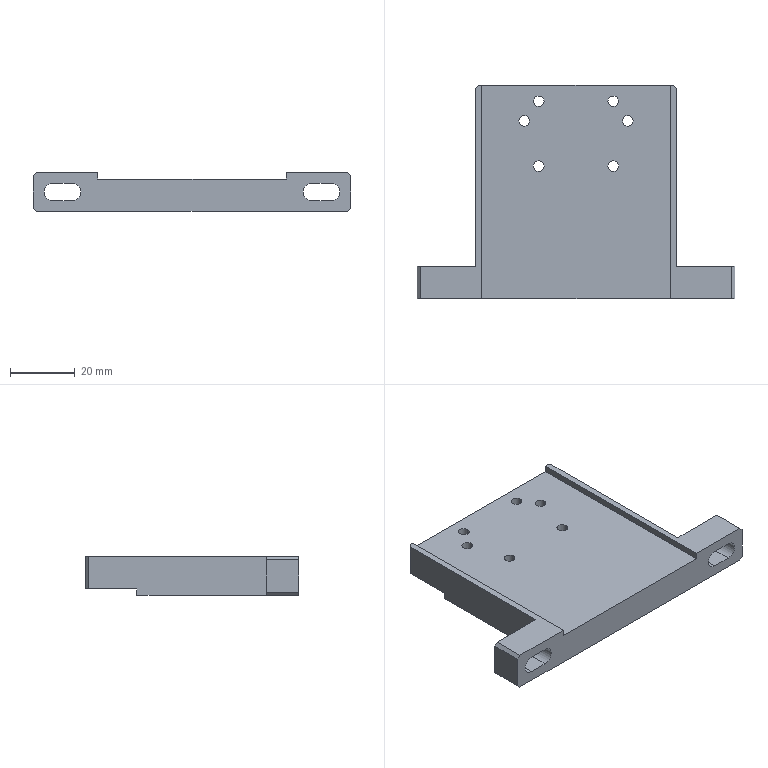Part | SolidWorks | features ICE 6, HoleWzd 4, Chamfer 2, Extrusion 1, MirrorPattern 1 | 1 solid | 42 faces | box 98 x 66 x 12 mm | volume 42190 mm3 | plane 26 | cylinder 16 | commonest cylinder face diameters 3.3 x12 5.4 x4
STEP:
#1=CARTESIAN_POINT('',(-13.15,8.,-6.));
#2=VERTEX_POINT('',#1);
#3=CARTESIAN_POINT('',(-9.85,8.,-6.));
#4=VERTEX_POINT('',#3);
#5=CARTESIAN_POINT('',(-11.5,8.,-6.));
#6=DIRECTION('',(0.,0.,1.));
#7=DIRECTION('',(1.,0.,0.));
#8=AXIS2_PLACEMENT_3D('',#5,#6,#7);
#9=CIRCLE('',#8,1.65);
#10=EDGE_CURVE('',#2,#4,#9,.T.);
#11=ORIENTED_EDGE('',*,*,#10,.F.);
#12=CARTESIAN_POINT('',(-13.15,8.,4.));
#13=VERTEX_POINT('',#12);
#14=CARTESIAN_POINT('',(-13.15,8.,4.));
#15=DIRECTION('',(0.,0.,1.));
#16=VECTOR('',#15,1000.);
#17=LINE('',#14,#16);
#18=EDGE_CURVE('',#2,#13,#17,.T.);
#19=ORIENTED_EDGE('',*,*,#18,.T.);
#20=CARTESIAN_POINT('',(-9.85,8.,4.));
#21=VERTEX_POINT('',#20);
#22=CARTESIAN_POINT('',(-11.5,8.,4.));
#23=DIRECTION('',(0.,0.,1.));
#24=DIRECTION('',(1.,0.,0.));
#25=AXIS2_PLACEMENT_3D('',#22,#23,#24);
#26=CIRCLE('',#25,1.65);
#27=EDGE_CURVE('',#13,#21,#26,.T.);
#28=ORIENTED_EDGE('',*,*,#27,.T.);
#29=CARTESIAN_POINT('',(-9.85,8.,4.));
#30=DIRECTION('',(0.,0.,1.));
#31=VECTOR('',#30,1000.);
#32=LINE('',#29,#31);
#33=EDGE_CURVE('',#4,#21,#32,.T.);
#34=ORIENTED_EDGE('',*,*,#33,.F.);
#35=EDGE_LOOP('',(#11,#19,#28,#34));
#36=FACE_OUTER_BOUND('',#35,.T.);
#37=CARTESIAN_POINT('',(-11.5,8.,4.));
#38=DIRECTION('',(0.,0.,1.));
#39=DIRECTION('',(1.,0.,0.));
#40=AXIS2_PLACEMENT_3D('',#37,#38,#39);
#41=CYLINDRICAL_SURFACE('',#40,1.65);
#42=ADVANCED_FACE('',(#36),#41,.F.);
#43=CARTESIAN_POINT('',(9.85,8.,-6.));
#44=VERTEX_POINT('',#43);
#45=CARTESIAN_POINT('',(13.15,8.,-6.));
#46=VERTEX_POINT('',#45);
#47=CARTESIAN_POINT('',(11.5,8.,-6.));
#48=DIRECTION('',(0.,0.,1.));
#49=DIRECTION('',(1.,0.,0.));
#50=AXIS2_PLACEMENT_3D('',#47,#48,#49);
#51=CIRCLE('',#50,1.65);
#52=EDGE_CURVE('',#44,#46,#51,.T.);
#53=ORIENTED_EDGE('',*,*,#52,.F.);
#54=CARTESIAN_POINT('',(9.85,8.,4.));
#55=VERTEX_POINT('',#54);
#56=CARTESIAN_POINT('',(9.85,8.,4.));
#57=DIRECTION('',(0.,0.,1.));
#58=VECTOR('',#57,1000.);
#59=LINE('',#56,#58);
#60=EDGE_CURVE('',#44,#55,#59,.T.);
#61=ORIENTED_EDGE('',*,*,#60,.T.);
#62=CARTESIAN_POINT('',(13.15,8.,4.));
#63=VERTEX_POINT('',#62);
#64=CARTESIAN_POINT('',(11.5,8.,4.));
#65=DIRECTION('',(0.,0.,1.));
#66=DIRECTION('',(1.,0.,0.));
#67=AXIS2_PLACEMENT_3D('',#64,#65,#66);
#68=CIRCLE('',#67,1.65);
#69=EDGE_CURVE('',#55,#63,#68,.T.);
#70=ORIENTED_EDGE('',*,*,#69,.T.);
#71=CARTESIAN_POINT('',(13.15,8.,4.));
#72=DIRECTION('',(0.,0.,1.));
#73=VECTOR('',#72,1000.);
#74=LINE('',#71,#73);
#75=EDGE_CURVE('',#46,#63,#74,.T.);
#76=ORIENTED_EDGE('',*,*,#75,.F.);
#77=EDGE_LOOP('',(#53,#61,#70,#76));
#78=FACE_OUTER_BOUND('',#77,.T.);
#79=CARTESIAN_POINT('',(11.5,8.,4.));
#80=DIRECTION('',(0.,0.,1.));
#81=DIRECTION('',(1.,0.,0.));
#82=AXIS2_PLACEMENT_3D('',#79,#80,#81);
#83=CYLINDRICAL_SURFACE('',#82,1.65);
#84=ADVANCED_FACE('',(#78),#83,.F.);
#85=CARTESIAN_POINT('',(14.35,22.,4.));
#86=VERTEX_POINT('',#85);
#87=CARTESIAN_POINT('',(17.65,22.,4.));
#88=VERTEX_POINT('',#87);
#89=CARTESIAN_POINT('',(16.,22.,4.));
#90=DIRECTION('',(0.,0.,1.));
#91=DIRECTION('',(1.,0.,0.));
#92=AXIS2_PLACEMENT_3D('',#89,#90,#91);
#93=CIRCLE('',#92,1.65);
#94=EDGE_CURVE('',#86,#88,#93,.T.);
#95=ORIENTED_EDGE('',*,*,#94,.T.);
#96=CARTESIAN_POINT('',(17.65,22.,-4.));
#97=VERTEX_POINT('',#96);
#98=CARTESIAN_POINT('',(17.65,22.,-6.));
#99=DIRECTION('',(0.,0.,-1.));
#100=VECTOR('',#99,1000.);
#101=LINE('',#98,#100);
#102=EDGE_CURVE('',#88,#97,#101,.T.);
#103=ORIENTED_EDGE('',*,*,#102,.T.);
#104=CARTESIAN_POINT('',(14.35,22.,-4.));
#105=VERTEX_POINT('',#104);
#106=CARTESIAN_POINT('',(16.,22.,-4.));
#107=DIRECTION('',(0.,0.,1.));
#108=DIRECTION('',(-1.,0.,0.));
#109=AXIS2_PLACEMENT_3D('',#106,#107,#108);
#110=CIRCLE('',#109,1.65);
#111=EDGE_CURVE('',#105,#97,#110,.T.);
#112=ORIENTED_EDGE('',*,*,#111,.F.);
#113=CARTESIAN_POINT('',(14.35,22.,-6.));
#114=DIRECTION('',(0.,0.,-1.));
#115=VECTOR('',#114,1000.);
#116=LINE('',#113,#115);
#117=EDGE_CURVE('',#86,#105,#116,.T.);
#118=ORIENTED_EDGE('',*,*,#117,.F.);
#119=EDGE_LOOP('',(#95,#103,#112,#118));
#120=FACE_OUTER_BOUND('',#119,.T.);
#121=CARTESIAN_POINT('',(16.,22.,-6.));
#122=DIRECTION('',(0.,0.,-1.));
#123=DIRECTION('',(-1.,0.,0.));
#124=AXIS2_PLACEMENT_3D('',#121,#122,#123);
#125=CYLINDRICAL_SURFACE('',#124,1.65);
#126=ADVANCED_FACE('',(#120),#125,.F.);
#127=CARTESIAN_POINT('',(-17.65,22.,4.));
#128=VERTEX_POINT('',#127);
#129=CARTESIAN_POINT('',(-14.35,22.,4.));
#130=VERTEX_POINT('',#129);
#131=CARTESIAN_POINT('',(-16.,22.,4.));
#132=DIRECTION('',(0.,0.,1.));
#133=DIRECTION('',(1.,0.,0.));
#134=AXIS2_PLACEMENT_3D('',#131,#132,#133);
#135=CIRCLE('',#134,1.65);
#136=EDGE_CURVE('',#128,#130,#135,.T.);
#137=ORIENTED_EDGE('',*,*,#136,.T.);
#138=CARTESIAN_POINT('',(-14.35,22.,-4.));
#139=VERTEX_POINT('',#138);
#140=CARTESIAN_POINT('',(-14.35,22.,-6.));
#141=DIRECTION('',(0.,0.,-1.));
#142=VECTOR('',#141,1000.);
#143=LINE('',#140,#142);
#144=EDGE_CURVE('',#130,#139,#143,.T.);
#145=ORIENTED_EDGE('',*,*,#144,.T.);
#146=CARTESIAN_POINT('',(-17.65,22.,-4.));
#147=VERTEX_POINT('',#146);
#148=CARTESIAN_POINT('',(-16.,22.,-4.));
#149=DIRECTION('',(0.,0.,1.));
#150=DIRECTION('',(-1.,0.,0.));
#151=AXIS2_PLACEMENT_3D('',#148,#149,#150);
#152=CIRCLE('',#151,1.65);
#153=EDGE_CURVE('',#147,#139,#152,.T.);
#154=ORIENTED_EDGE('',*,*,#153,.F.);
#155=CARTESIAN_POINT('',(-17.65,22.,-6.));
#156=DIRECTION('',(0.,0.,-1.));
#157=VECTOR('',#156,1000.);
#158=LINE('',#155,#157);
#159=EDGE_CURVE('',#128,#147,#158,.T.);
#160=ORIENTED_EDGE('',*,*,#159,.F.);
#161=EDGE_LOOP('',(#137,#145,#154,#160));
#162=FACE_OUTER_BOUND('',#161,.T.);
#163=CARTESIAN_POINT('',(-16.,22.,-6.));
#164=DIRECTION('',(0.,0.,-1.));
#165=DIRECTION('',(-1.,0.,0.));
#166=AXIS2_PLACEMENT_3D('',#163,#164,#165);
#167=CYLINDRICAL_SURFACE('',#166,1.65);
#168=ADVANCED_FACE('',(#162),#167,.F.);
#169=CARTESIAN_POINT('',(-13.15,28.,-4.));
#170=VERTEX_POINT('',#169);
#171=CARTESIAN_POINT('',(-9.85,28.,-4.));
#172=VERTEX_POINT('',#171);
#173=CARTESIAN_POINT('',(-11.5,28.,-4.));
#174=DIRECTION('',(0.,0.,1.));
#175=DIRECTION('',(-1.,0.,0.));
#176=AXIS2_PLACEMENT_3D('',#173,#174,#175);
#177=CIRCLE('',#176,1.65);
#178=EDGE_CURVE('',#170,#172,#177,.T.);
#179=ORIENTED_EDGE('',*,*,#178,.F.);
#180=CARTESIAN_POINT('',(-13.15,28.,4.));
#181=VERTEX_POINT('',#180);
#182=CARTESIAN_POINT('',(-13.15,28.,4.));
#183=DIRECTION('',(0.,0.,1.));
#184=VECTOR('',#183,1000.);
#185=LINE('',#182,#184);
#186=EDGE_CURVE('',#170,#181,#185,.T.);
#187=ORIENTED_EDGE('',*,*,#186,.T.);
#188=CARTESIAN_POINT('',(-9.85,28.,4.));
#189=VERTEX_POINT('',#188);
#190=CARTESIAN_POINT('',(-11.5,28.,4.));
#191=DIRECTION('',(0.,0.,1.));
#192=DIRECTION('',(1.,0.,0.));
#193=AXIS2_PLACEMENT_3D('',#190,#191,#192);
#194=CIRCLE('',#193,1.65);
#195=EDGE_CURVE('',#181,#189,#194,.T.);
#196=ORIENTED_EDGE('',*,*,#195,.T.);
#197=CARTESIAN_POINT('',(-9.85,28.,4.));
#198=DIRECTION('',(0.,0.,1.));
#199=VECTOR('',#198,1000.);
#200=LINE('',#197,#199);
#201=EDGE_CURVE('',#172,#189,#200,.T.);
#202=ORIENTED_EDGE('',*,*,#201,.F.);
#203=EDGE_LOOP('',(#179,#187,#196,#202));
#204=FACE_OUTER_BOUND('',#203,.T.);
#205=CARTESIAN_POINT('',(-11.5,28.,4.));
#206=DIRECTION('',(0.,0.,1.));
#207=DIRECTION('',(1.,0.,0.));
#208=AXIS2_PLACEMENT_3D('',#205,#206,#207);
#209=CYLINDRICAL_SURFACE('',#208,1.65);
#210=ADVANCED_FACE('',(#204),#209,.F.);
#211=CARTESIAN_POINT('',(9.85,28.,-4.));
#212=VERTEX_POINT('',#211);
#213=CARTESIAN_POINT('',(13.15,28.,-4.));
#214=VERTEX_POINT('',#213);
#215=CARTESIAN_POINT('',(11.5,28.,-4.));
#216=DIRECTION('',(0.,0.,1.));
#217=DIRECTION('',(-1.,0.,0.));
#218=AXIS2_PLACEMENT_3D('',#215,#216,#217);
#219=CIRCLE('',#218,1.65);
#220=EDGE_CURVE('',#212,#214,#219,.T.);
#221=ORIENTED_EDGE('',*,*,#220,.F.);
#222=CARTESIAN_POINT('',(9.85,28.,4.));
#223=VERTEX_POINT('',#222);
#224=CARTESIAN_POINT('',(9.85,28.,4.));
#225=DIRECTION('',(0.,0.,1.));
#226=VECTOR('',#225,1000.);
#227=LINE('',#224,#226);
#228=EDGE_CURVE('',#212,#223,#227,.T.);
#229=ORIENTED_EDGE('',*,*,#228,.T.);
#230=CARTESIAN_POINT('',(13.15,28.,4.));
#231=VERTEX_POINT('',#230);
#232=CARTESIAN_POINT('',(11.5,28.,4.));
#233=DIRECTION('',(0.,0.,1.));
#234=DIRECTION('',(1.,0.,0.));
#235=AXIS2_PLACEMENT_3D('',#232,#233,#234);
#236=CIRCLE('',#235,1.65);
#237=EDGE_CURVE('',#223,#231,#236,.T.);
#238=ORIENTED_EDGE('',*,*,#237,.T.);
#239=CARTESIAN_POINT('',(13.15,28.,4.));
#240=DIRECTION('',(0.,0.,1.));
#241=VECTOR('',#240,1000.);
#242=LINE('',#239,#241);
#243=EDGE_CURVE('',#214,#231,#242,.T.);
#244=ORIENTED_EDGE('',*,*,#243,.F.);
#245=EDGE_LOOP('',(#221,#229,#238,#244));
#246=FACE_OUTER_BOUND('',#245,.T.);
#247=CARTESIAN_POINT('',(11.5,28.,4.));
#248=DIRECTION('',(0.,0.,1.));
#249=DIRECTION('',(1.,0.,0.));
#250=AXIS2_PLACEMENT_3D('',#247,#248,#249);
#251=CYLINDRICAL_SURFACE('',#250,1.65);
#252=ADVANCED_FACE('',(#246),#251,.F.);
#253=CARTESIAN_POINT('',(-30.,33.,-4.));
#254=VERTEX_POINT('',#253);
#255=CARTESIAN_POINT('',(30.,33.,-4.));
#256=VERTEX_POINT('',#255);
#257=CARTESIAN_POINT('',(-31.,33.,-4.));
#258=DIRECTION('',(1.,0.,0.));
#259=VECTOR('',#258,1000.);
#260=LINE('',#257,#259);
#261=EDGE_CURVE('',#254,#256,#260,.T.);
#262=ORIENTED_EDGE('',*,*,#261,.F.);
#263=CARTESIAN_POINT('',(-30.,33.,6.));
#264=VERTEX_POINT('',#263);
#265=CARTESIAN_POINT('',(-30.,33.,6.));
#266=DIRECTION('',(0.,0.,1.));
#267=VECTOR('',#266,1000.);
#268=LINE('',#265,#267);
#269=EDGE_CURVE('',#254,#264,#268,.T.);
#270=ORIENTED_EDGE('',*,*,#269,.T.);
#271=CARTESIAN_POINT('',(-29.05,33.,6.));
#272=VERTEX_POINT('',#271);
#273=CARTESIAN_POINT('',(-31.,33.,6.));
#274=DIRECTION('',(-1.,0.,0.));
#275=VECTOR('',#274,1000.);
#276=LINE('',#273,#275);
#277=EDGE_CURVE('',#272,#264,#276,.T.);
#278=ORIENTED_EDGE('',*,*,#277,.F.);
#279=CARTESIAN_POINT('',(-29.05,33.,4.));
#280=VERTEX_POINT('',#279);
#281=CARTESIAN_POINT('',(-29.05,33.,6.));
#282=DIRECTION('',(0.,0.,-1.));
#283=VECTOR('',#282,1000.);
#284=LINE('',#281,#283);
#285=EDGE_CURVE('',#272,#280,#284,.T.);
#286=ORIENTED_EDGE('',*,*,#285,.T.);
#287=CARTESIAN_POINT('',(29.05,33.,4.));
#288=VERTEX_POINT('',#287);
#289=CARTESIAN_POINT('',(-31.,33.,4.));
#290=DIRECTION('',(-1.,0.,0.));
#291=VECTOR('',#290,1000.);
#292=LINE('',#289,#291);
#293=EDGE_CURVE('',#288,#280,#292,.T.);
#294=ORIENTED_EDGE('',*,*,#293,.F.);
#295=CARTESIAN_POINT('',(29.05,33.,6.));
#296=VERTEX_POINT('',#295);
#297=CARTESIAN_POINT('',(29.05,33.,6.));
#298=DIRECTION('',(0.,0.,1.));
#299=VECTOR('',#298,1000.);
#300=LINE('',#297,#299);
#301=EDGE_CURVE('',#288,#296,#300,.T.);
#302=ORIENTED_EDGE('',*,*,#301,.T.);
#303=CARTESIAN_POINT('',(30.,33.,6.));
#304=VERTEX_POINT('',#303);
#305=CARTESIAN_POINT('',(-31.,33.,6.));
#306=DIRECTION('',(-1.,0.,0.));
#307=VECTOR('',#306,1000.);
#308=LINE('',#305,#307);
#309=EDGE_CURVE('',#304,#296,#308,.T.);
#310=ORIENTED_EDGE('',*,*,#309,.F.);
#311=CARTESIAN_POINT('',(30.,33.,6.));
#312=DIRECTION('',(0.,0.,-1.));
#313=VECTOR('',#312,1000.);
#314=LINE('',#311,#313);
#315=EDGE_CURVE('',#304,#256,#314,.T.);
#316=ORIENTED_EDGE('',*,*,#315,.T.);
#317=EDGE_LOOP('',(#262,#270,#278,#286,#294,#302,#310,#316));
#318=FACE_OUTER_BOUND('',#317,.T.);
#319=CARTESIAN_POINT('',(-31.,33.,6.));
#320=DIRECTION('',(0.,-1.,0.));
#321=DIRECTION('',(0.,0.,-1.));
#322=AXIS2_PLACEMENT_3D('',#319,#320,#321);
#323=PLANE('',#322);
#324=ADVANCED_FACE('',(#318),#323,.F.);
#325=ORIENTED_EDGE('',*,*,#228,.F.);
#326=CARTESIAN_POINT('',(11.5,28.,-4.));
#327=DIRECTION('',(0.,0.,1.));
#328=DIRECTION('',(-1.,0.,0.));
#329=AXIS2_PLACEMENT_3D('',#326,#327,#328);
#330=CIRCLE('',#329,1.65);
#331=EDGE_CURVE('',#214,#212,#330,.T.);
#332=ORIENTED_EDGE('',*,*,#331,.F.);
#333=ORIENTED_EDGE('',*,*,#243,.T.);
#334=CARTESIAN_POINT('',(11.5,28.,4.));
#335=DIRECTION('',(0.,0.,1.));
#336=DIRECTION('',(1.,0.,0.));
#337=AXIS2_PLACEMENT_3D('',#334,#335,#336);
#338=CIRCLE('',#337,1.65);
#339=EDGE_CURVE('',#231,#223,#338,.T.);
#340=ORIENTED_EDGE('',*,*,#339,.T.);
#341=EDGE_LOOP('',(#325,#332,#333,#340));
#342=FACE_OUTER_BOUND('',#341,.T.);
#343=CARTESIAN_POINT('',(11.5,28.,4.));
#344=DIRECTION('',(0.,0.,1.));
#345=DIRECTION('',(1.,0.,0.));
#346=AXIS2_PLACEMENT_3D('',#343,#344,#345);
#347=CYLINDRICAL_SURFACE('',#346,1.65);
#348=ADVANCED_FACE('',(#342),#347,.F.);
#349=ORIENTED_EDGE('',*,*,#186,.F.);
#350=CARTESIAN_POINT('',(-11.5,28.,-4.));
#351=DIRECTION('',(0.,0.,1.));
#352=DIRECTION('',(-1.,0.,0.));
#353=AXIS2_PLACEMENT_3D('',#350,#351,#352);
#354=CIRCLE('',#353,1.65);
#355=EDGE_CURVE('',#172,#170,#354,.T.);
#356=ORIENTED_EDGE('',*,*,#355,.F.);
#357=ORIENTED_EDGE('',*,*,#201,.T.);
#358=CARTESIAN_POINT('',(-11.5,28.,4.));
#359=DIRECTION('',(0.,0.,1.));
#360=DIRECTION('',(1.,0.,0.));
#361=AXIS2_PLACEMENT_3D('',#358,#359,#360);
#362=CIRCLE('',#361,1.65);
#363=EDGE_CURVE('',#189,#181,#362,.T.);
#364=ORIENTED_EDGE('',*,*,#363,.T.);
#365=EDGE_LOOP('',(#349,#356,#357,#364));
#366=FACE_OUTER_BOUND('',#365,.T.);
#367=CARTESIAN_POINT('',(-11.5,28.,4.));
#368=DIRECTION('',(0.,0.,1.));
#369=DIRECTION('',(1.,0.,0.));
#370=AXIS2_PLACEMENT_3D('',#367,#368,#369);
#371=CYLINDRICAL_SURFACE('',#370,1.65);
#372=ADVANCED_FACE('',(#366),#371,.F.);
#373=ORIENTED_EDGE('',*,*,#144,.F.);
#374=CARTESIAN_POINT('',(-16.,22.,4.));
#375=DIRECTION('',(0.,0.,1.));
#376=DIRECTION('',(1.,0.,0.));
#377=AXIS2_PLACEMENT_3D('',#374,#375,#376);
#378=CIRCLE('',#377,1.65);
#379=EDGE_CURVE('',#130,#128,#378,.T.);
#380=ORIENTED_EDGE('',*,*,#379,.T.);
#381=ORIENTED_EDGE('',*,*,#159,.T.);
#382=CARTESIAN_POINT('',(-16.,22.,-4.));
#383=DIRECTION('',(0.,0.,1.));
#384=DIRECTION('',(-1.,0.,0.));
#385=AXIS2_PLACEMENT_3D('',#382,#383,#384);
#386=CIRCLE('',#385,1.65);
#387=EDGE_CURVE('',#139,#147,#386,.T.);
#388=ORIENTED_EDGE('',*,*,#387,.F.);
#389=EDGE_LOOP('',(#373,#380,#381,#388));
#390=FACE_OUTER_BOUND('',#389,.T.);
#391=CARTESIAN_POINT('',(-16.,22.,-6.));
#392=DIRECTION('',(0.,0.,-1.));
#393=DIRECTION('',(-1.,0.,0.));
#394=AXIS2_PLACEMENT_3D('',#391,#392,#393);
#395=CYLINDRICAL_SURFACE('',#394,1.65);
#396=ADVANCED_FACE('',(#390),#395,.F.);
#397=ORIENTED_EDGE('',*,*,#102,.F.);
#398=CARTESIAN_POINT('',(16.,22.,4.));
#399=DIRECTION('',(0.,0.,1.));
#400=DIRECTION('',(1.,0.,0.));
#401=AXIS2_PLACEMENT_3D('',#398,#399,#400);
#402=CIRCLE('',#401,1.65);
#403=EDGE_CURVE('',#88,#86,#402,.T.);
#404=ORIENTED_EDGE('',*,*,#403,.T.);
#405=ORIENTED_EDGE('',*,*,#117,.T.);
#406=CARTESIAN_POINT('',(16.,22.,-4.));
#407=DIRECTION('',(0.,0.,1.));
#408=DIRECTION('',(-1.,0.,0.));
#409=AXIS2_PLACEMENT_3D('',#406,#407,#408);
#410=CIRCLE('',#409,1.65);
#411=EDGE_CURVE('',#97,#105,#410,.T.);
#412=ORIENTED_EDGE('',*,*,#411,.F.);
#413=EDGE_LOOP('',(#397,#404,#405,#412));
#414=FACE_OUTER_BOUND('',#413,.T.);
#415=CARTESIAN_POINT('',(16.,22.,-6.));
#416=DIRECTION('',(0.,0.,-1.));
#417=DIRECTION('',(-1.,0.,0.));
#418=AXIS2_PLACEMENT_3D('',#415,#416,#417);
#419=CYLINDRICAL_SURFACE('',#418,1.65);
#420=ADVANCED_FACE('',(#414),#419,.F.);
#421=ORIENTED_EDGE('',*,*,#277,.T.);
#422=CARTESIAN_POINT('',(-31.,32.,6.));
#423=VERTEX_POINT('',#422);
#424=CARTESIAN_POINT('',(-31.5,31.5,6.));
#425=DIRECTION('',(-0.7071,-0.7071,0.));
#426=VECTOR('',#425,1000.);
#427=LINE('',#424,#426);
#428=EDGE_CURVE('',#264,#423,#427,.T.);
#429=ORIENTED_EDGE('',*,*,#428,.T.);
#430=CARTESIAN_POINT('',(-31.,-23.,6.));
#431=VERTEX_POINT('',#430);
#432=CARTESIAN_POINT('',(-31.,33.,6.));
#433=DIRECTION('',(0.,-1.,0.));
#434=VECTOR('',#433,1000.);
#435=LINE('',#432,#434);
#436=EDGE_CURVE('',#423,#431,#435,.T.);
#437=ORIENTED_EDGE('',*,*,#436,.T.);
#438=CARTESIAN_POINT('',(-48.,-23.,6.));
#439=VERTEX_POINT('',#438);
#440=CARTESIAN_POINT('',(-49.,-23.,6.));
#441=DIRECTION('',(-1.,0.,0.));
#442=VECTOR('',#441,1000.);
#443=LINE('',#440,#442);
#444=EDGE_CURVE('',#431,#439,#443,.T.);
#445=ORIENTED_EDGE('',*,*,#444,.T.);
#446=CARTESIAN_POINT('',(-48.,-33.,6.));
#447=VERTEX_POINT('',#446);
#448=CARTESIAN_POINT('',(-48.,0.,6.));
#449=DIRECTION('',(0.,-1.,0.));
#450=VECTOR('',#449,1000.);
#451=LINE('',#448,#450);
#452=EDGE_CURVE('',#439,#447,#451,.T.);
#453=ORIENTED_EDGE('',*,*,#452,.T.);
#454=CARTESIAN_POINT('',(-29.05,-33.,6.));
#455=VERTEX_POINT('',#454);
#456=CARTESIAN_POINT('',(-31.,-33.,6.));
#457=DIRECTION('',(1.,0.,0.));
#458=VECTOR('',#457,1000.);
#459=LINE('',#456,#458);
#460=EDGE_CURVE('',#447,#455,#459,.T.);
#461=ORIENTED_EDGE('',*,*,#460,.T.);
#462=CARTESIAN_POINT('',(-29.05,0.,6.));
#463=DIRECTION('',(0.,-1.,0.));
#464=VECTOR('',#463,1000.);
#465=LINE('',#462,#464);
#466=EDGE_CURVE('',#272,#455,#465,.T.);
#467=ORIENTED_EDGE('',*,*,#466,.F.);
#468=EDGE_LOOP('',(#421,#429,#437,#445,#453,#461,#467));
#469=FACE_OUTER_BOUND('',#468,.T.);
#470=CARTESIAN_POINT('',(0.,0.,6.));
#471=DIRECTION('',(0.,0.,1.));
#472=DIRECTION('',(1.,0.,0.));
#473=AXIS2_PLACEMENT_3D('',#470,#471,#472);
#474=PLANE('',#473);
#475=ADVANCED_FACE('',(#469),#474,.T.);
#476=CARTESIAN_POINT('',(-49.,-33.,5.));
#477=VERTEX_POINT('',#476);
#478=CARTESIAN_POINT('',(-49.,-33.,-5.));
#479=VERTEX_POINT('',#478);
#480=CARTESIAN_POINT('',(-49.,-33.,6.));
#481=DIRECTION('',(0.,0.,-1.));
#482=VECTOR('',#481,1000.);
#483=LINE('',#480,#482);
#484=EDGE_CURVE('',#477,#479,#483,.T.);
#485=ORIENTED_EDGE('',*,*,#484,.T.);
#486=CARTESIAN_POINT('',(-48.,-33.,-6.));
#487=VERTEX_POINT('',#486);
#488=CARTESIAN_POINT('',(-49.,-33.,-5.));
#489=DIRECTION('',(0.7071,0.,-0.7071));
#490=VECTOR('',#489,1000.);
#491=LINE('',#488,#490);
#492=EDGE_CURVE('',#479,#487,#491,.T.);
#493=ORIENTED_EDGE('',*,*,#492,.T.);
#494=CARTESIAN_POINT('',(48.,-33.,-6.));
#495=VERTEX_POINT('',#494);
#496=CARTESIAN_POINT('',(-31.,-33.,-6.));
#497=DIRECTION('',(1.,0.,0.));
#498=VECTOR('',#497,1000.);
#499=LINE('',#496,#498);
#500=EDGE_CURVE('',#487,#495,#499,.T.);
#501=ORIENTED_EDGE('',*,*,#500,.T.);
#502=CARTESIAN_POINT('',(49.,-33.,-5.));
#503=VERTEX_POINT('',#502);
#504=CARTESIAN_POINT('',(48.,-33.,-6.));
#505=DIRECTION('',(0.7071,0.,0.7071));
#506=VECTOR('',#505,1000.);
#507=LINE('',#504,#506);
#508=EDGE_CURVE('',#495,#503,#507,.T.);
#509=ORIENTED_EDGE('',*,*,#508,.T.);
#510=CARTESIAN_POINT('',(49.,-33.,5.));
#511=VERTEX_POINT('',#510);
#512=CARTESIAN_POINT('',(49.,-33.,6.));
#513=DIRECTION('',(0.,0.,1.));
#514=VECTOR('',#513,1000.);
#515=LINE('',#512,#514);
#516=EDGE_CURVE('',#503,#511,#515,.T.);
#517=ORIENTED_EDGE('',*,*,#516,.T.);
#518=CARTESIAN_POINT('',(48.,-33.,6.));
#519=VERTEX_POINT('',#518);
#520=CARTESIAN_POINT('',(49.,-33.,5.));
#521=DIRECTION('',(-0.7071,0.,0.7071));
#522=VECTOR('',#521,1000.);
#523=LINE('',#520,#522);
#524=EDGE_CURVE('',#511,#519,#523,.T.);
#525=ORIENTED_EDGE('',*,*,#524,.T.);
#526=CARTESIAN_POINT('',(29.05,-33.,6.));
#527=VERTEX_POINT('',#526);
#528=CARTESIAN_POINT('',(-31.,-33.,6.));
#529=DIRECTION('',(1.,0.,0.));
#530=VECTOR('',#529,1000.);
#531=LINE('',#528,#530);
#532=EDGE_CURVE('',#527,#519,#531,.T.);
#533=ORIENTED_EDGE('',*,*,#532,.F.);
#534=CARTESIAN_POINT('',(29.05,-33.,4.));
#535=VERTEX_POINT('',#534);
#536=CARTESIAN_POINT('',(29.05,-33.,6.));
#537=DIRECTION('',(0.,0.,-1.));
#538=VECTOR('',#537,1000.);
#539=LINE('',#536,#538);
#540=EDGE_CURVE('',#527,#535,#539,.T.);
#541=ORIENTED_EDGE('',*,*,#540,.T.);
#542=CARTESIAN_POINT('',(-29.05,-33.,4.));
#543=VERTEX_POINT('',#542);
#544=CARTESIAN_POINT('',(-31.,-33.,4.));
#545=DIRECTION('',(1.,0.,0.));
#546=VECTOR('',#545,1000.);
#547=LINE('',#544,#546);
#548=EDGE_CURVE('',#543,#535,#547,.T.);
#549=ORIENTED_EDGE('',*,*,#548,.F.);
#550=CARTESIAN_POINT('',(-29.05,-33.,6.));
#551=DIRECTION('',(0.,0.,1.));
#552=VECTOR('',#551,1000.);
#553=LINE('',#550,#552);
#554=EDGE_CURVE('',#543,#455,#553,.T.);
#555=ORIENTED_EDGE('',*,*,#554,.T.);
#556=ORIENTED_EDGE('',*,*,#460,.F.);
#557=CARTESIAN_POINT('',(-48.,-33.,6.));
#558=DIRECTION('',(-0.7071,0.,-0.7071));
#559=VECTOR('',#558,1000.);
#560=LINE('',#557,#559);
#561=EDGE_CURVE('',#447,#477,#560,.T.);
#562=ORIENTED_EDGE('',*,*,#561,.T.);
#563=EDGE_LOOP('',(#485,#493,#501,#509,#517,#525,#533,#541,#549,#555,#556,#562));
#564=FACE_OUTER_BOUND('',#563,.T.);
#565=CARTESIAN_POINT('',(-37.,-33.,-2.7));
#566=VERTEX_POINT('',#565);
#567=CARTESIAN_POINT('',(-43.,-33.,-2.7));
#568=VERTEX_POINT('',#567);
#569=CARTESIAN_POINT('',(-43.,-33.,-2.7));
#570=DIRECTION('',(-1.,0.,0.));
#571=VECTOR('',#570,1000.);
#572=LINE('',#569,#571);
#573=EDGE_CURVE('',#566,#568,#572,.T.);
#574=ORIENTED_EDGE('',*,*,#573,.T.);
#575=CARTESIAN_POINT('',(-43.,-33.,2.7));
#576=VERTEX_POINT('',#575);
#577=CARTESIAN_POINT('',(-43.,-33.,0.));
#578=DIRECTION('',(0.,1.,0.));
#579=DIRECTION('',(0.,0.,1.));
#580=AXIS2_PLACEMENT_3D('',#577,#578,#579);
#581=CIRCLE('',#580,2.7);
#582=EDGE_CURVE('',#568,#576,#581,.T.);
#583=ORIENTED_EDGE('',*,*,#582,.T.);
#584=CARTESIAN_POINT('',(-37.,-33.,2.7));
#585=VERTEX_POINT('',#584);
#586=CARTESIAN_POINT('',(-43.,-33.,2.7));
#587=DIRECTION('',(1.,0.,0.));
#588=VECTOR('',#587,1000.);
#589=LINE('',#586,#588);
#590=EDGE_CURVE('',#576,#585,#589,.T.);
#591=ORIENTED_EDGE('',*,*,#590,.T.);
#592=CARTESIAN_POINT('',(-37.,-33.,0.));
#593=DIRECTION('',(0.,1.,0.));
#594=DIRECTION('',(0.,0.,1.));
#595=AXIS2_PLACEMENT_3D('',#592,#593,#594);
#596=CIRCLE('',#595,2.7);
#597=EDGE_CURVE('',#585,#566,#596,.T.);
#598=ORIENTED_EDGE('',*,*,#597,.T.);
#599=EDGE_LOOP('',(#574,#583,#591,#598));
#600=FACE_BOUND('',#599,.T.);
#601=CARTESIAN_POINT('',(43.,-33.,-2.7));
#602=VERTEX_POINT('',#601);
#603=CARTESIAN_POINT('',(43.,-33.,2.7));
#604=VERTEX_POINT('',#603);
#605=CARTESIAN_POINT('',(43.,-33.,0.));
#606=DIRECTION('',(0.,-1.,0.));
#607=DIRECTION('',(0.,0.,1.));
#608=AXIS2_PLACEMENT_3D('',#605,#606,#607);
#609=CIRCLE('',#608,2.7);
#610=EDGE_CURVE('',#602,#604,#609,.T.);
#611=ORIENTED_EDGE('',*,*,#610,.F.);
#612=CARTESIAN_POINT('',(37.,-33.,-2.7));
#613=VERTEX_POINT('',#612);
#614=CARTESIAN_POINT('',(43.,-33.,-2.7));
#615=DIRECTION('',(1.,0.,0.));
#616=VECTOR('',#615,1000.);
#617=LINE('',#614,#616);
#618=EDGE_CURVE('',#613,#602,#617,.T.);
#619=ORIENTED_EDGE('',*,*,#618,.F.);
#620=CARTESIAN_POINT('',(37.,-33.,2.7));
#621=VERTEX_POINT('',#620);
#622=CARTESIAN_POINT('',(37.,-33.,0.));
#623=DIRECTION('',(0.,-1.,0.));
#624=DIRECTION('',(0.,0.,1.));
#625=AXIS2_PLACEMENT_3D('',#622,#623,#624);
#626=CIRCLE('',#625,2.7);
#627=EDGE_CURVE('',#621,#613,#626,.T.);
#628=ORIENTED_EDGE('',*,*,#627,.F.);
#629=CARTESIAN_POINT('',(43.,-33.,2.7));
#630=DIRECTION('',(-1.,0.,0.));
#631=VECTOR('',#630,1000.);
#632=LINE('',#629,#631);
#633=EDGE_CURVE('',#604,#621,#632,.T.);
#634=ORIENTED_EDGE('',*,*,#633,.F.);
#635=EDGE_LOOP('',(#611,#619,#628,#634));
#636=FACE_BOUND('',#635,.T.);
#637=CARTESIAN_POINT('',(-31.,-33.,6.));
#638=DIRECTION('',(0.,1.,0.));
#639=DIRECTION('',(0.,0.,1.));
#640=AXIS2_PLACEMENT_3D('',#637,#638,#639);
#641=PLANE('',#640);
#642=ADVANCED_FACE('',(#564,#600,#636),#641,.F.);
#643=CARTESIAN_POINT('',(49.,-23.,-5.));
#644=VERTEX_POINT('',#643);
#645=CARTESIAN_POINT('',(49.,-23.,5.));
#646=VERTEX_POINT('',#645);
#647=CARTESIAN_POINT('',(49.,-23.,6.));
#648=DIRECTION('',(0.,0.,1.));
#649=VECTOR('',#648,1000.);
#650=LINE('',#647,#649);
#651=EDGE_CURVE('',#644,#646,#650,.T.);
#652=ORIENTED_EDGE('',*,*,#651,.F.);
#653=CARTESIAN_POINT('',(48.,-23.,-6.));
#654=VERTEX_POINT('',#653);
#655=CARTESIAN_POINT('',(48.,-23.,-6.));
#656=DIRECTION('',(-0.7071,0.,-0.7071));
#657=VECTOR('',#656,1000.);
#658=LINE('',#655,#657);
#659=EDGE_CURVE('',#644,#654,#658,.T.);
#660=ORIENTED_EDGE('',*,*,#659,.T.);
#661=CARTESIAN_POINT('',(31.,-23.,-6.));
#662=VERTEX_POINT('',#661);
#663=CARTESIAN_POINT('',(-49.,-23.,-6.));
#664=DIRECTION('',(1.,0.,0.));
#665=VECTOR('',#664,1000.);
#666=LINE('',#663,#665);
#667=EDGE_CURVE('',#662,#654,#666,.T.);
#668=ORIENTED_EDGE('',*,*,#667,.F.);
#669=CARTESIAN_POINT('',(31.,-23.,6.));
#670=VERTEX_POINT('',#669);
#671=CARTESIAN_POINT('',(31.,-23.,6.));
#672=DIRECTION('',(0.,0.,1.));
#673=VECTOR('',#672,1000.);
#674=LINE('',#671,#673);
#675=EDGE_CURVE('',#662,#670,#674,.T.);
#676=ORIENTED_EDGE('',*,*,#675,.T.);
#677=CARTESIAN_POINT('',(48.,-23.,6.));
#678=VERTEX_POINT('',#677);
#679=CARTESIAN_POINT('',(-49.,-23.,6.));
#680=DIRECTION('',(-1.,0.,0.));
#681=VECTOR('',#680,1000.);
#682=LINE('',#679,#681);
#683=EDGE_CURVE('',#678,#670,#682,.T.);
#684=ORIENTED_EDGE('',*,*,#683,.F.);
#685=CARTESIAN_POINT('',(49.,-23.,5.));
#686=DIRECTION('',(0.7071,0.,-0.7071));
#687=VECTOR('',#686,1000.);
#688=LINE('',#685,#687);
#689=EDGE_CURVE('',#678,#646,#688,.T.);
#690=ORIENTED_EDGE('',*,*,#689,.T.);
#691=EDGE_LOOP('',(#652,#660,#668,#676,#684,#690));
#692=FACE_OUTER_BOUND('',#691,.T.);
#693=CARTESIAN_POINT('',(43.,-23.,-2.7));
#694=VERTEX_POINT('',#693);
#695=CARTESIAN_POINT('',(43.,-23.,2.7));
#696=VERTEX_POINT('',#695);
#697=CARTESIAN_POINT('',(43.,-23.,0.));
#698=DIRECTION('',(0.,-1.,0.));
#699=DIRECTION('',(0.,0.,1.));
#700=AXIS2_PLACEMENT_3D('',#697,#698,#699);
#701=CIRCLE('',#700,2.7);
#702=EDGE_CURVE('',#694,#696,#701,.T.);
#703=ORIENTED_EDGE('',*,*,#702,.T.);
#704=CARTESIAN_POINT('',(37.,-23.,2.7));
#705=VERTEX_POINT('',#704);
#706=CARTESIAN_POINT('',(43.,-23.,2.7));
#707=DIRECTION('',(-1.,0.,0.));
#708=VECTOR('',#707,1000.);
#709=LINE('',#706,#708);
#710=EDGE_CURVE('',#696,#705,#709,.T.);
#711=ORIENTED_EDGE('',*,*,#710,.T.);
#712=CARTESIAN_POINT('',(37.,-23.,-2.7));
#713=VERTEX_POINT('',#712);
#714=CARTESIAN_POINT('',(37.,-23.,0.));
#715=DIRECTION('',(0.,-1.,0.));
#716=DIRECTION('',(0.,0.,1.));
#717=AXIS2_PLACEMENT_3D('',#714,#715,#716);
#718=CIRCLE('',#717,2.7);
#719=EDGE_CURVE('',#705,#713,#718,.T.);
#720=ORIENTED_EDGE('',*,*,#719,.T.);
#721=CARTESIAN_POINT('',(43.,-23.,-2.7));
#722=DIRECTION('',(1.,0.,0.));
#723=VECTOR('',#722,1000.);
#724=LINE('',#721,#723);
#725=EDGE_CURVE('',#713,#694,#724,.T.);
#726=ORIENTED_EDGE('',*,*,#725,.T.);
#727=EDGE_LOOP('',(#703,#711,#720,#726));
#728=FACE_BOUND('',#727,.T.);
#729=CARTESIAN_POINT('',(0.,-23.,0.));
#730=DIRECTION('',(0.,-1.,0.));
#731=DIRECTION('',(0.,0.,-1.));
#732=AXIS2_PLACEMENT_3D('',#729,#730,#731);
#733=PLANE('',#732);
#734=ADVANCED_FACE('',(#692,#728),#733,.F.);
#735=CARTESIAN_POINT('',(31.,32.,-4.));
#736=VERTEX_POINT('',#735);
#737=CARTESIAN_POINT('',(31.,17.,-4.));
#738=VERTEX_POINT('',#737);
#739=CARTESIAN_POINT('',(31.,33.,-4.));
#740=DIRECTION('',(0.,-1.,0.));
#741=VECTOR('',#740,1000.);
#742=LINE('',#739,#741);
#743=EDGE_CURVE('',#736,#738,#742,.T.);
#744=ORIENTED_EDGE('',*,*,#743,.F.);
#745=CARTESIAN_POINT('',(31.,32.,6.));
#746=VERTEX_POINT('',#745);
#747=CARTESIAN_POINT('',(31.,32.,6.));
#748=DIRECTION('',(0.,0.,1.));
#749=VECTOR('',#748,1000.);
#750=LINE('',#747,#749);
#751=EDGE_CURVE('',#736,#746,#750,.T.);
#752=ORIENTED_EDGE('',*,*,#751,.T.);
#753=CARTESIAN_POINT('',(31.,33.,6.));
#754=DIRECTION('',(0.,1.,0.));
#755=VECTOR('',#754,1000.);
#756=LINE('',#753,#755);
#757=EDGE_CURVE('',#670,#746,#756,.T.);
#758=ORIENTED_EDGE('',*,*,#757,.F.);
#759=ORIENTED_EDGE('',*,*,#675,.F.);
#760=CARTESIAN_POINT('',(31.,17.,-6.));
#761=VERTEX_POINT('',#760);
#762=CARTESIAN_POINT('',(31.,33.,-6.));
#763=DIRECTION('',(0.,1.,0.));
#764=VECTOR('',#763,1000.);
#765=LINE('',#762,#764);
#766=EDGE_CURVE('',#662,#761,#765,.T.);
#767=ORIENTED_EDGE('',*,*,#766,.T.);
#768=CARTESIAN_POINT('',(31.,17.,6.));
#769=DIRECTION('',(0.,0.,1.));
#770=VECTOR('',#769,1000.);
#771=LINE('',#768,#770);
#772=EDGE_CURVE('',#761,#738,#771,.T.);
#773=ORIENTED_EDGE('',*,*,#772,.T.);
#774=EDGE_LOOP('',(#744,#752,#758,#759,#767,#773));
#775=FACE_OUTER_BOUND('',#774,.T.);
#776=CARTESIAN_POINT('',(31.,33.,6.));
#777=DIRECTION('',(-1.,0.,0.));
#778=DIRECTION('',(0.,-1.,0.));
#779=AXIS2_PLACEMENT_3D('',#776,#777,#778);
#780=PLANE('',#779);
#781=ADVANCED_FACE('',(#775),#780,.F.);
#782=ORIENTED_EDGE('',*,*,#436,.F.);
#783=CARTESIAN_POINT('',(-31.,32.,-4.));
#784=VERTEX_POINT('',#783);
#785=CARTESIAN_POINT('',(-31.,32.,6.));
#786=DIRECTION('',(0.,0.,-1.));
#787=VECTOR('',#786,1000.);
#788=LINE('',#785,#787);
#789=EDGE_CURVE('',#423,#784,#788,.T.);
#790=ORIENTED_EDGE('',*,*,#789,.T.);
#791=CARTESIAN_POINT('',(-31.,17.,-4.));
#792=VERTEX_POINT('',#791);
#793=CARTESIAN_POINT('',(-31.,33.,-4.));
#794=DIRECTION('',(0.,1.,0.));
#795=VECTOR('',#794,1000.);
#796=LINE('',#793,#795);
#797=EDGE_CURVE('',#792,#784,#796,.T.);
#798=ORIENTED_EDGE('',*,*,#797,.F.);
#799=CARTESIAN_POINT('',(-31.,17.,-6.));
#800=VERTEX_POINT('',#799);
#801=CARTESIAN_POINT('',(-31.,17.,6.));
#802=DIRECTION('',(0.,0.,-1.));
#803=VECTOR('',#802,1000.);
#804=LINE('',#801,#803);
#805=EDGE_CURVE('',#792,#800,#804,.T.);
#806=ORIENTED_EDGE('',*,*,#805,.T.);
#807=CARTESIAN_POINT('',(-31.,-23.,-6.));
#808=VERTEX_POINT('',#807);
#809=CARTESIAN_POINT('',(-31.,33.,-6.));
#810=DIRECTION('',(0.,-1.,0.));
#811=VECTOR('',#810,1000.);
#812=LINE('',#809,#811);
#813=EDGE_CURVE('',#800,#808,#812,.T.);
#814=ORIENTED_EDGE('',*,*,#813,.T.);
#815=CARTESIAN_POINT('',(-31.,-23.,6.));
#816=DIRECTION('',(0.,0.,-1.));
#817=VECTOR('',#816,1000.);
#818=LINE('',#815,#817);
#819=EDGE_CURVE('',#431,#808,#818,.T.);
#820=ORIENTED_EDGE('',*,*,#819,.F.);
#821=EDGE_LOOP('',(#782,#790,#798,#806,#814,#820));
#822=FACE_OUTER_BOUND('',#821,.T.);
#823=CARTESIAN_POINT('',(-31.,33.,6.));
#824=DIRECTION('',(1.,0.,0.));
#825=DIRECTION('',(0.,1.,0.));
#826=AXIS2_PLACEMENT_3D('',#823,#824,#825);
#827=PLANE('',#826);
#828=ADVANCED_FACE('',(#822),#827,.F.);
#829=CARTESIAN_POINT('',(-29.05,56.846,4.));
#830=DIRECTION('',(0.,-1.,0.));
#831=VECTOR('',#830,1000.);
#832=LINE('',#829,#831);
#833=EDGE_CURVE('',#280,#543,#832,.T.);
#834=ORIENTED_EDGE('',*,*,#833,.T.);
#835=ORIENTED_EDGE('',*,*,#548,.T.);
#836=CARTESIAN_POINT('',(29.05,56.846,4.));
#837=DIRECTION('',(0.,1.,0.));
#838=VECTOR('',#837,1000.);
#839=LINE('',#836,#838);
#840=EDGE_CURVE('',#535,#288,#839,.T.);
#841=ORIENTED_EDGE('',*,*,#840,.T.);
#842=ORIENTED_EDGE('',*,*,#293,.T.);
#843=EDGE_LOOP('',(#834,#835,#841,#842));
#844=FACE_OUTER_BOUND('',#843,.T.);
#845=CARTESIAN_POINT('',(11.5,8.,4.));
#846=DIRECTION('',(0.,0.,1.));
#847=DIRECTION('',(1.,0.,0.));
#848=AXIS2_PLACEMENT_3D('',#845,#846,#847);
#849=CIRCLE('',#848,1.65);
#850=EDGE_CURVE('',#63,#55,#849,.T.);
#851=ORIENTED_EDGE('',*,*,#850,.F.);
#852=ORIENTED_EDGE('',*,*,#69,.F.);
#853=EDGE_LOOP('',(#851,#852));
#854=FACE_BOUND('',#853,.T.);
#855=CARTESIAN_POINT('',(-11.5,8.,4.));
#856=DIRECTION('',(0.,0.,1.));
#857=DIRECTION('',(1.,0.,0.));
#858=AXIS2_PLACEMENT_3D('',#855,#856,#857);
#859=CIRCLE('',#858,1.65);
#860=EDGE_CURVE('',#21,#13,#859,.T.);
#861=ORIENTED_EDGE('',*,*,#860,.F.);
#862=ORIENTED_EDGE('',*,*,#27,.F.);
#863=EDGE_LOOP('',(#861,#862));
#864=FACE_BOUND('',#863,.T.);
#865=ORIENTED_EDGE('',*,*,#339,.F.);
#866=ORIENTED_EDGE('',*,*,#237,.F.);
#867=EDGE_LOOP('',(#865,#866));
#868=FACE_BOUND('',#867,.T.);
#869=ORIENTED_EDGE('',*,*,#363,.F.);
#870=ORIENTED_EDGE('',*,*,#195,.F.);
#871=EDGE_LOOP('',(#869,#870));
#872=FACE_BOUND('',#871,.T.);
#873=ORIENTED_EDGE('',*,*,#136,.F.);
#874=ORIENTED_EDGE('',*,*,#379,.F.);
#875=EDGE_LOOP('',(#873,#874));
#876=FACE_BOUND('',#875,.T.);
#877=ORIENTED_EDGE('',*,*,#94,.F.);
#878=ORIENTED_EDGE('',*,*,#403,.F.);
#879=EDGE_LOOP('',(#877,#878));
#880=FACE_BOUND('',#879,.T.);
#881=CARTESIAN_POINT('',(0.,0.,4.));
#882=DIRECTION('',(0.,0.,1.));
#883=DIRECTION('',(1.,0.,0.));
#884=AXIS2_PLACEMENT_3D('',#881,#882,#883);
#885=PLANE('',#884);
#886=ADVANCED_FACE('',(#844,#854,#864,#868,#872,#876,#880),#885,.T.);
#887=ORIENTED_EDGE('',*,*,#301,.F.);
#888=ORIENTED_EDGE('',*,*,#840,.F.);
#889=ORIENTED_EDGE('',*,*,#540,.F.);
#890=CARTESIAN_POINT('',(29.05,0.,6.));
#891=DIRECTION('',(0.,1.,0.));
#892=VECTOR('',#891,1000.);
#893=LINE('',#890,#892);
#894=EDGE_CURVE('',#527,#296,#893,.T.);
#895=ORIENTED_EDGE('',*,*,#894,.T.);
#896=EDGE_LOOP('',(#887,#888,#889,#895));
#897=FACE_OUTER_BOUND('',#896,.T.);
#898=CARTESIAN_POINT('',(29.05,56.846,4.));
#899=DIRECTION('',(1.,0.,0.));
#900=DIRECTION('',(0.,1.,0.));
#901=AXIS2_PLACEMENT_3D('',#898,#899,#900);
#902=PLANE('',#901);
#903=ADVANCED_FACE('',(#897),#902,.F.);
#904=ORIENTED_EDGE('',*,*,#466,.T.);
#905=ORIENTED_EDGE('',*,*,#554,.F.);
#906=ORIENTED_EDGE('',*,*,#833,.F.);
#907=ORIENTED_EDGE('',*,*,#285,.F.);
#908=EDGE_LOOP('',(#904,#905,#906,#907));
#909=FACE_OUTER_BOUND('',#908,.T.);
#910=CARTESIAN_POINT('',(-29.05,56.846,4.));
#911=DIRECTION('',(-1.,0.,0.));
#912=DIRECTION('',(0.,-1.,0.));
#913=AXIS2_PLACEMENT_3D('',#910,#911,#912);
#914=PLANE('',#913);
#915=ADVANCED_FACE('',(#909),#914,.F.);
#916=ORIENTED_EDGE('',*,*,#757,.T.);
#917=CARTESIAN_POINT('',(31.5,31.5,6.));
#918=DIRECTION('',(-0.7071,0.7071,0.));
#919=VECTOR('',#918,1000.);
#920=LINE('',#917,#919);
#921=EDGE_CURVE('',#746,#304,#920,.T.);
#922=ORIENTED_EDGE('',*,*,#921,.T.);
#923=ORIENTED_EDGE('',*,*,#309,.T.);
#924=ORIENTED_EDGE('',*,*,#894,.F.);
#925=ORIENTED_EDGE('',*,*,#532,.T.);
#926=CARTESIAN_POINT('',(48.,0.,6.));
#927=DIRECTION('',(0.,1.,0.));
#928=VECTOR('',#927,1000.);
#929=LINE('',#926,#928);
#930=EDGE_CURVE('',#519,#678,#929,.T.);
#931=ORIENTED_EDGE('',*,*,#930,.T.);
#932=ORIENTED_EDGE('',*,*,#683,.T.);
#933=EDGE_LOOP('',(#916,#922,#923,#924,#925,#931,#932));
#934=FACE_OUTER_BOUND('',#933,.T.);
#935=CARTESIAN_POINT('',(0.,0.,6.));
#936=DIRECTION('',(0.,0.,1.));
#937=DIRECTION('',(1.,0.,0.));
#938=AXIS2_PLACEMENT_3D('',#935,#936,#937);
#939=PLANE('',#938);
#940=ADVANCED_FACE('',(#934),#939,.T.);
#941=ORIENTED_EDGE('',*,*,#500,.F.);
#942=CARTESIAN_POINT('',(-48.,-23.,-6.));
#943=VERTEX_POINT('',#942);
#944=CARTESIAN_POINT('',(-48.,-23.,-6.));
#945=DIRECTION('',(0.,1.,0.));
#946=VECTOR('',#945,1000.);
#947=LINE('',#944,#946);
#948=EDGE_CURVE('',#487,#943,#947,.T.);
#949=ORIENTED_EDGE('',*,*,#948,.T.);
#950=CARTESIAN_POINT('',(-49.,-23.,-6.));
#951=DIRECTION('',(1.,0.,0.));
#952=VECTOR('',#951,1000.);
#953=LINE('',#950,#952);
#954=EDGE_CURVE('',#943,#808,#953,.T.);
#955=ORIENTED_EDGE('',*,*,#954,.T.);
#956=ORIENTED_EDGE('',*,*,#813,.F.);
#957=CARTESIAN_POINT('',(71.901,17.,-6.));
#958=DIRECTION('',(-1.,0.,0.));
#959=VECTOR('',#958,1000.);
#960=LINE('',#957,#959);
#961=EDGE_CURVE('',#761,#800,#960,.T.);
#962=ORIENTED_EDGE('',*,*,#961,.F.);
#963=ORIENTED_EDGE('',*,*,#766,.F.);
#964=ORIENTED_EDGE('',*,*,#667,.T.);
#965=CARTESIAN_POINT('',(48.,-33.,-6.));
#966=DIRECTION('',(0.,-1.,0.));
#967=VECTOR('',#966,1000.);
#968=LINE('',#965,#967);
#969=EDGE_CURVE('',#654,#495,#968,.T.);
#970=ORIENTED_EDGE('',*,*,#969,.T.);
#971=EDGE_LOOP('',(#941,#949,#955,#956,#962,#963,#964,#970));
#972=FACE_OUTER_BOUND('',#971,.T.);
#973=CARTESIAN_POINT('',(11.5,8.,-6.));
#974=DIRECTION('',(0.,0.,1.));
#975=DIRECTION('',(1.,0.,0.));
#976=AXIS2_PLACEMENT_3D('',#973,#974,#975);
#977=CIRCLE('',#976,1.65);
#978=EDGE_CURVE('',#46,#44,#977,.T.);
#979=ORIENTED_EDGE('',*,*,#978,.T.);
#980=ORIENTED_EDGE('',*,*,#52,.T.);
#981=EDGE_LOOP('',(#979,#980));
#982=FACE_BOUND('',#981,.T.);
#983=CARTESIAN_POINT('',(-11.5,8.,-6.));
#984=DIRECTION('',(0.,0.,1.));
#985=DIRECTION('',(1.,0.,0.));
#986=AXIS2_PLACEMENT_3D('',#983,#984,#985);
#987=CIRCLE('',#986,1.65);
#988=EDGE_CURVE('',#4,#2,#987,.T.);
#989=ORIENTED_EDGE('',*,*,#988,.T.);
#990=ORIENTED_EDGE('',*,*,#10,.T.);
#991=EDGE_LOOP('',(#989,#990));
#992=FACE_BOUND('',#991,.T.);
#993=CARTESIAN_POINT('',(0.,0.,-6.));
#994=DIRECTION('',(0.,0.,1.));
#995=DIRECTION('',(1.,0.,0.));
#996=AXIS2_PLACEMENT_3D('',#993,#994,#995);
#997=PLANE('',#996);
#998=ADVANCED_FACE('',(#972,#982,#992),#997,.F.);
#999=ORIENTED_EDGE('',*,*,#60,.F.);
#1000=ORIENTED_EDGE('',*,*,#978,.F.);
#1001=ORIENTED_EDGE('',*,*,#75,.T.);
#1002=ORIENTED_EDGE('',*,*,#850,.T.);
#1003=EDGE_LOOP('',(#999,#1000,#1001,#1002));
#1004=FACE_OUTER_BOUND('',#1003,.T.);
#1005=CARTESIAN_POINT('',(11.5,8.,4.));
#1006=DIRECTION('',(0.,0.,1.));
#1007=DIRECTION('',(1.,0.,0.));
#1008=AXIS2_PLACEMENT_3D('',#1005,#1006,#1007);
#1009=CYLINDRICAL_SURFACE('',#1008,1.65);
#1010=ADVANCED_FACE('',(#1004),#1009,.F.);
#1011=ORIENTED_EDGE('',*,*,#18,.F.);
#1012=ORIENTED_EDGE('',*,*,#988,.F.);
#1013=ORIENTED_EDGE('',*,*,#33,.T.);
#1014=ORIENTED_EDGE('',*,*,#860,.T.);
#1015=EDGE_LOOP('',(#1011,#1012,#1013,#1014));
#1016=FACE_OUTER_BOUND('',#1015,.T.);
#1017=CARTESIAN_POINT('',(-11.5,8.,4.));
#1018=DIRECTION('',(0.,0.,1.));
#1019=DIRECTION('',(1.,0.,0.));
#1020=AXIS2_PLACEMENT_3D('',#1017,#1018,#1019);
#1021=CYLINDRICAL_SURFACE('',#1020,1.65);
#1022=ADVANCED_FACE('',(#1016),#1021,.F.);
#1023=CARTESIAN_POINT('',(-49.,-23.,5.));
#1024=VERTEX_POINT('',#1023);
#1025=CARTESIAN_POINT('',(-49.,-23.,-5.));
#1026=VERTEX_POINT('',#1025);
#1027=CARTESIAN_POINT('',(-49.,-23.,6.));
#1028=DIRECTION('',(0.,0.,-1.));
#1029=VECTOR('',#1028,1000.);
#1030=LINE('',#1027,#1029);
#1031=EDGE_CURVE('',#1024,#1026,#1030,.T.);
#1032=ORIENTED_EDGE('',*,*,#1031,.T.);
#1033=CARTESIAN_POINT('',(-49.,-33.,-5.));
#1034=DIRECTION('',(0.,-1.,0.));
#1035=VECTOR('',#1034,1000.);
#1036=LINE('',#1033,#1035);
#1037=EDGE_CURVE('',#1026,#479,#1036,.T.);
#1038=ORIENTED_EDGE('',*,*,#1037,.T.);
#1039=ORIENTED_EDGE('',*,*,#484,.F.);
#1040=CARTESIAN_POINT('',(-49.,-23.,5.));
#1041=DIRECTION('',(0.,1.,0.));
#1042=VECTOR('',#1041,1000.);
#1043=LINE('',#1040,#1042);
#1044=EDGE_CURVE('',#477,#1024,#1043,.T.);
#1045=ORIENTED_EDGE('',*,*,#1044,.T.);
#1046=EDGE_LOOP('',(#1032,#1038,#1039,#1045));
#1047=FACE_OUTER_BOUND('',#1046,.T.);
#1048=CARTESIAN_POINT('',(-49.,-23.,6.));
#1049=DIRECTION('',(-1.,0.,0.));
#1050=DIRECTION('',(0.,0.,1.));
#1051=AXIS2_PLACEMENT_3D('',#1048,#1049,#1050);
#1052=PLANE('',#1051);
#1053=ADVANCED_FACE('',(#1047),#1052,.T.);
#1054=CARTESIAN_POINT('',(-43.,-23.,2.7));
#1055=VERTEX_POINT('',#1054);
#1056=CARTESIAN_POINT('',(-37.,-23.,2.7));
#1057=VERTEX_POINT('',#1056);
#1058=CARTESIAN_POINT('',(-43.,-23.,2.7));
#1059=DIRECTION('',(1.,0.,0.));
#1060=VECTOR('',#1059,1000.);
#1061=LINE('',#1058,#1060);
#1062=EDGE_CURVE('',#1055,#1057,#1061,.T.);
#1063=ORIENTED_EDGE('',*,*,#1062,.F.);
#1064=CARTESIAN_POINT('',(-43.,-23.,-2.7));
#1065=VERTEX_POINT('',#1064);
#1066=CARTESIAN_POINT('',(-43.,-23.,0.));
#1067=DIRECTION('',(0.,1.,0.));
#1068=DIRECTION('',(0.,0.,1.));
#1069=AXIS2_PLACEMENT_3D('',#1066,#1067,#1068);
#1070=CIRCLE('',#1069,2.7);
#1071=EDGE_CURVE('',#1065,#1055,#1070,.T.);
#1072=ORIENTED_EDGE('',*,*,#1071,.F.);
#1073=CARTESIAN_POINT('',(-37.,-23.,-2.7));
#1074=VERTEX_POINT('',#1073);
#1075=CARTESIAN_POINT('',(-43.,-23.,-2.7));
#1076=DIRECTION('',(-1.,0.,0.));
#1077=VECTOR('',#1076,1000.);
#1078=LINE('',#1075,#1077);
#1079=EDGE_CURVE('',#1074,#1065,#1078,.T.);
#1080=ORIENTED_EDGE('',*,*,#1079,.F.);
#1081=CARTESIAN_POINT('',(-37.,-23.,0.));
#1082=DIRECTION('',(0.,1.,0.));
#1083=DIRECTION('',(0.,0.,1.));
#1084=AXIS2_PLACEMENT_3D('',#1081,#1082,#1083);
#1085=CIRCLE('',#1084,2.7);
#1086=EDGE_CURVE('',#1057,#1074,#1085,.T.);
#1087=ORIENTED_EDGE('',*,*,#1086,.F.);
#1088=EDGE_LOOP('',(#1063,#1072,#1080,#1087));
#1089=FACE_BOUND('',#1088,.T.);
#1090=ORIENTED_EDGE('',*,*,#954,.F.);
#1091=CARTESIAN_POINT('',(-49.,-23.,-5.));
#1092=DIRECTION('',(-0.7071,0.,0.7071));
#1093=VECTOR('',#1092,1000.);
#1094=LINE('',#1091,#1093);
#1095=EDGE_CURVE('',#943,#1026,#1094,.T.);
#1096=ORIENTED_EDGE('',*,*,#1095,.T.);
#1097=ORIENTED_EDGE('',*,*,#1031,.F.);
#1098=CARTESIAN_POINT('',(-48.,-23.,6.));
#1099=DIRECTION('',(0.7071,0.,0.7071));
#1100=VECTOR('',#1099,1000.);
#1101=LINE('',#1098,#1100);
#1102=EDGE_CURVE('',#1024,#439,#1101,.T.);
#1103=ORIENTED_EDGE('',*,*,#1102,.T.);
#1104=ORIENTED_EDGE('',*,*,#444,.F.);
#1105=ORIENTED_EDGE('',*,*,#819,.T.);
#1106=EDGE_LOOP('',(#1090,#1096,#1097,#1103,#1104,#1105));
#1107=FACE_OUTER_BOUND('',#1106,.T.);
#1108=CARTESIAN_POINT('',(0.,-23.,0.));
#1109=DIRECTION('',(0.,-1.,0.));
#1110=DIRECTION('',(0.,0.,-1.));
#1111=AXIS2_PLACEMENT_3D('',#1108,#1109,#1110);
#1112=PLANE('',#1111);
#1113=ADVANCED_FACE('',(#1089,#1107),#1112,.F.);
#1114=ORIENTED_EDGE('',*,*,#516,.F.);
#1115=CARTESIAN_POINT('',(49.,-23.,-5.));
#1116=DIRECTION('',(0.,1.,0.));
#1117=VECTOR('',#1116,1000.);
#1118=LINE('',#1115,#1117);
#1119=EDGE_CURVE('',#503,#644,#1118,.T.);
#1120=ORIENTED_EDGE('',*,*,#1119,.T.);
#1121=ORIENTED_EDGE('',*,*,#651,.T.);
#1122=CARTESIAN_POINT('',(49.,-23.,5.));
#1123=DIRECTION('',(0.,-1.,0.));
#1124=VECTOR('',#1123,1000.);
#1125=LINE('',#1122,#1124);
#1126=EDGE_CURVE('',#646,#511,#1125,.T.);
#1127=ORIENTED_EDGE('',*,*,#1126,.T.);
#1128=EDGE_LOOP('',(#1114,#1120,#1121,#1127));
#1129=FACE_OUTER_BOUND('',#1128,.T.);
#1130=CARTESIAN_POINT('',(49.,-23.,6.));
#1131=DIRECTION('',(1.,0.,0.));
#1132=DIRECTION('',(0.,0.,-1.));
#1133=AXIS2_PLACEMENT_3D('',#1130,#1131,#1132);
#1134=PLANE('',#1133);
#1135=ADVANCED_FACE('',(#1129),#1134,.T.);
#1136=ORIENTED_EDGE('',*,*,#1071,.T.);
#1137=CARTESIAN_POINT('',(-43.,-33.,2.7));
#1138=DIRECTION('',(0.,1.,0.));
#1139=VECTOR('',#1138,1000.);
#1140=LINE('',#1137,#1139);
#1141=EDGE_CURVE('',#576,#1055,#1140,.T.);
#1142=ORIENTED_EDGE('',*,*,#1141,.F.);
#1143=ORIENTED_EDGE('',*,*,#582,.F.);
#1144=CARTESIAN_POINT('',(-43.,-33.,-2.7));
#1145=DIRECTION('',(0.,1.,0.));
#1146=VECTOR('',#1145,1000.);
#1147=LINE('',#1144,#1146);
#1148=EDGE_CURVE('',#568,#1065,#1147,.T.);
#1149=ORIENTED_EDGE('',*,*,#1148,.T.);
#1150=EDGE_LOOP('',(#1136,#1142,#1143,#1149));
#1151=FACE_OUTER_BOUND('',#1150,.T.);
#1152=CARTESIAN_POINT('',(-43.,-33.,0.));
#1153=DIRECTION('',(0.,1.,0.));
#1154=DIRECTION('',(0.,0.,1.));
#1155=AXIS2_PLACEMENT_3D('',#1152,#1153,#1154);
#1156=CYLINDRICAL_SURFACE('',#1155,2.7);
#1157=ADVANCED_FACE('',(#1151),#1156,.F.);
#1158=ORIENTED_EDGE('',*,*,#1079,.T.);
#1159=ORIENTED_EDGE('',*,*,#1148,.F.);
#1160=ORIENTED_EDGE('',*,*,#573,.F.);
#1161=CARTESIAN_POINT('',(-37.,-33.,-2.7));
#1162=DIRECTION('',(0.,1.,0.));
#1163=VECTOR('',#1162,1000.);
#1164=LINE('',#1161,#1163);
#1165=EDGE_CURVE('',#566,#1074,#1164,.T.);
#1166=ORIENTED_EDGE('',*,*,#1165,.T.);
#1167=EDGE_LOOP('',(#1158,#1159,#1160,#1166));
#1168=FACE_OUTER_BOUND('',#1167,.T.);
#1169=CARTESIAN_POINT('',(-43.,-33.,-2.7));
#1170=DIRECTION('',(0.,0.,-1.));
#1171=DIRECTION('',(-1.,0.,0.));
#1172=AXIS2_PLACEMENT_3D('',#1169,#1170,#1171);
#1173=PLANE('',#1172);
#1174=ADVANCED_FACE('',(#1168),#1173,.F.);
#1175=ORIENTED_EDGE('',*,*,#1086,.T.);
#1176=ORIENTED_EDGE('',*,*,#1165,.F.);
#1177=ORIENTED_EDGE('',*,*,#597,.F.);
#1178=CARTESIAN_POINT('',(-37.,-33.,2.7));
#1179=DIRECTION('',(0.,1.,0.));
#1180=VECTOR('',#1179,1000.);
#1181=LINE('',#1178,#1180);
#1182=EDGE_CURVE('',#585,#1057,#1181,.T.);
#1183=ORIENTED_EDGE('',*,*,#1182,.T.);
#1184=EDGE_LOOP('',(#1175,#1176,#1177,#1183));
#1185=FACE_OUTER_BOUND('',#1184,.T.);
#1186=CARTESIAN_POINT('',(-37.,-33.,0.));
#1187=DIRECTION('',(0.,1.,0.));
#1188=DIRECTION('',(0.,0.,1.));
#1189=AXIS2_PLACEMENT_3D('',#1186,#1187,#1188);
#1190=CYLINDRICAL_SURFACE('',#1189,2.7);
#1191=ADVANCED_FACE('',(#1185),#1190,.F.);
#1192=ORIENTED_EDGE('',*,*,#1062,.T.);
#1193=ORIENTED_EDGE('',*,*,#1182,.F.);
#1194=ORIENTED_EDGE('',*,*,#590,.F.);
#1195=ORIENTED_EDGE('',*,*,#1141,.T.);
#1196=EDGE_LOOP('',(#1192,#1193,#1194,#1195));
#1197=FACE_OUTER_BOUND('',#1196,.T.);
#1198=CARTESIAN_POINT('',(-43.,-33.,2.7));
#1199=DIRECTION('',(0.,0.,1.));
#1200=DIRECTION('',(1.,0.,0.));
#1201=AXIS2_PLACEMENT_3D('',#1198,#1199,#1200);
#1202=PLANE('',#1201);
#1203=ADVANCED_FACE('',(#1197),#1202,.F.);
#1204=ORIENTED_EDGE('',*,*,#702,.F.);
#1205=CARTESIAN_POINT('',(43.,-33.,-2.7));
#1206=DIRECTION('',(0.,1.,0.));
#1207=VECTOR('',#1206,1000.);
#1208=LINE('',#1205,#1207);
#1209=EDGE_CURVE('',#602,#694,#1208,.T.);
#1210=ORIENTED_EDGE('',*,*,#1209,.F.);
#1211=ORIENTED_EDGE('',*,*,#610,.T.);
#1212=CARTESIAN_POINT('',(43.,-33.,2.7));
#1213=DIRECTION('',(0.,1.,0.));
#1214=VECTOR('',#1213,1000.);
#1215=LINE('',#1212,#1214);
#1216=EDGE_CURVE('',#604,#696,#1215,.T.);
#1217=ORIENTED_EDGE('',*,*,#1216,.T.);
#1218=EDGE_LOOP('',(#1204,#1210,#1211,#1217));
#1219=FACE_OUTER_BOUND('',#1218,.T.);
#1220=CARTESIAN_POINT('',(43.,-33.,0.));
#1221=DIRECTION('',(0.,1.,0.));
#1222=DIRECTION('',(0.,0.,1.));
#1223=AXIS2_PLACEMENT_3D('',#1220,#1221,#1222);
#1224=CYLINDRICAL_SURFACE('',#1223,2.7);
#1225=ADVANCED_FACE('',(#1219),#1224,.F.);
#1226=ORIENTED_EDGE('',*,*,#710,.F.);
#1227=ORIENTED_EDGE('',*,*,#1216,.F.);
#1228=ORIENTED_EDGE('',*,*,#633,.T.);
#1229=CARTESIAN_POINT('',(37.,-33.,2.7));
#1230=DIRECTION('',(0.,1.,0.));
#1231=VECTOR('',#1230,1000.);
#1232=LINE('',#1229,#1231);
#1233=EDGE_CURVE('',#621,#705,#1232,.T.);
#1234=ORIENTED_EDGE('',*,*,#1233,.T.);
#1235=EDGE_LOOP('',(#1226,#1227,#1228,#1234));
#1236=FACE_OUTER_BOUND('',#1235,.T.);
#1237=CARTESIAN_POINT('',(43.,-33.,2.7));
#1238=DIRECTION('',(0.,0.,-1.));
#1239=DIRECTION('',(-1.,0.,0.));
#1240=AXIS2_PLACEMENT_3D('',#1237,#1238,#1239);
#1241=PLANE('',#1240);
#1242=ADVANCED_FACE('',(#1236),#1241,.T.);
#1243=ORIENTED_EDGE('',*,*,#719,.F.);
#1244=ORIENTED_EDGE('',*,*,#1233,.F.);
#1245=ORIENTED_EDGE('',*,*,#627,.T.);
#1246=CARTESIAN_POINT('',(37.,-33.,-2.7));
#1247=DIRECTION('',(0.,1.,0.));
#1248=VECTOR('',#1247,1000.);
#1249=LINE('',#1246,#1248);
#1250=EDGE_CURVE('',#613,#713,#1249,.T.);
#1251=ORIENTED_EDGE('',*,*,#1250,.T.);
#1252=EDGE_LOOP('',(#1243,#1244,#1245,#1251));
#1253=FACE_OUTER_BOUND('',#1252,.T.);
#1254=CARTESIAN_POINT('',(37.,-33.,0.));
#1255=DIRECTION('',(0.,1.,0.));
#1256=DIRECTION('',(0.,0.,1.));
#1257=AXIS2_PLACEMENT_3D('',#1254,#1255,#1256);
#1258=CYLINDRICAL_SURFACE('',#1257,2.7);
#1259=ADVANCED_FACE('',(#1253),#1258,.F.);
#1260=ORIENTED_EDGE('',*,*,#725,.F.);
#1261=ORIENTED_EDGE('',*,*,#1250,.F.);
#1262=ORIENTED_EDGE('',*,*,#618,.T.);
#1263=ORIENTED_EDGE('',*,*,#1209,.T.);
#1264=EDGE_LOOP('',(#1260,#1261,#1262,#1263));
#1265=FACE_OUTER_BOUND('',#1264,.T.);
#1266=CARTESIAN_POINT('',(43.,-33.,-2.7));
#1267=DIRECTION('',(0.,0.,1.));
#1268=DIRECTION('',(1.,0.,0.));
#1269=AXIS2_PLACEMENT_3D('',#1266,#1267,#1268);
#1270=PLANE('',#1269);
#1271=ADVANCED_FACE('',(#1265),#1270,.T.);
#1272=ORIENTED_EDGE('',*,*,#961,.T.);
#1273=ORIENTED_EDGE('',*,*,#805,.F.);
#1274=CARTESIAN_POINT('',(71.901,17.,-4.));
#1275=DIRECTION('',(-1.,0.,0.));
#1276=VECTOR('',#1275,1000.);
#1277=LINE('',#1274,#1276);
#1278=EDGE_CURVE('',#738,#792,#1277,.T.);
#1279=ORIENTED_EDGE('',*,*,#1278,.F.);
#1280=ORIENTED_EDGE('',*,*,#772,.F.);
#1281=EDGE_LOOP('',(#1272,#1273,#1279,#1280));
#1282=FACE_OUTER_BOUND('',#1281,.T.);
#1283=CARTESIAN_POINT('',(71.901,17.,-4.));
#1284=DIRECTION('',(0.,-1.,0.));
#1285=DIRECTION('',(0.,0.,-1.));
#1286=AXIS2_PLACEMENT_3D('',#1283,#1284,#1285);
#1287=PLANE('',#1286);
#1288=ADVANCED_FACE('',(#1282),#1287,.F.);
#1289=ORIENTED_EDGE('',*,*,#331,.T.);
#1290=ORIENTED_EDGE('',*,*,#220,.T.);
#1291=EDGE_LOOP('',(#1289,#1290));
#1292=FACE_BOUND('',#1291,.T.);
#1293=ORIENTED_EDGE('',*,*,#153,.T.);
#1294=ORIENTED_EDGE('',*,*,#387,.T.);
#1295=EDGE_LOOP('',(#1293,#1294));
#1296=FACE_BOUND('',#1295,.T.);
#1297=ORIENTED_EDGE('',*,*,#111,.T.);
#1298=ORIENTED_EDGE('',*,*,#411,.T.);
#1299=EDGE_LOOP('',(#1297,#1298));
#1300=FACE_BOUND('',#1299,.T.);
#1301=ORIENTED_EDGE('',*,*,#355,.T.);
#1302=ORIENTED_EDGE('',*,*,#178,.T.);
#1303=EDGE_LOOP('',(#1301,#1302));
#1304=FACE_BOUND('',#1303,.T.);
#1305=ORIENTED_EDGE('',*,*,#797,.T.);
#1306=CARTESIAN_POINT('',(-31.5,31.5,-4.));
#1307=DIRECTION('',(0.7071,0.7071,0.));
#1308=VECTOR('',#1307,1000.);
#1309=LINE('',#1306,#1308);
#1310=EDGE_CURVE('',#784,#254,#1309,.T.);
#1311=ORIENTED_EDGE('',*,*,#1310,.T.);
#1312=ORIENTED_EDGE('',*,*,#261,.T.);
#1313=CARTESIAN_POINT('',(31.5,31.5,-4.));
#1314=DIRECTION('',(0.7071,-0.7071,0.));
#1315=VECTOR('',#1314,1000.);
#1316=LINE('',#1313,#1315);
#1317=EDGE_CURVE('',#256,#736,#1316,.T.);
#1318=ORIENTED_EDGE('',*,*,#1317,.T.);
#1319=ORIENTED_EDGE('',*,*,#743,.T.);
#1320=ORIENTED_EDGE('',*,*,#1278,.T.);
#1321=EDGE_LOOP('',(#1305,#1311,#1312,#1318,#1319,#1320));
#1322=FACE_OUTER_BOUND('',#1321,.T.);
#1323=CARTESIAN_POINT('',(0.,0.,-4.));
#1324=DIRECTION('',(0.,0.,-1.));
#1325=DIRECTION('',(-1.,0.,0.));
#1326=AXIS2_PLACEMENT_3D('',#1323,#1324,#1325);
#1327=PLANE('',#1326);
#1328=ADVANCED_FACE('',(#1292,#1296,#1300,#1304,#1322),#1327,.T.);
#1329=ORIENTED_EDGE('',*,*,#1095,.F.);
#1330=ORIENTED_EDGE('',*,*,#948,.F.);
#1331=ORIENTED_EDGE('',*,*,#492,.F.);
#1332=ORIENTED_EDGE('',*,*,#1037,.F.);
#1333=EDGE_LOOP('',(#1329,#1330,#1331,#1332));
#1334=FACE_OUTER_BOUND('',#1333,.T.);
#1335=CARTESIAN_POINT('',(-49.,-23.,-5.));
#1336=DIRECTION('',(-0.7071,0.,-0.7071));
#1337=DIRECTION('',(0.,1.,0.));
#1338=AXIS2_PLACEMENT_3D('',#1335,#1336,#1337);
#1339=PLANE('',#1338);
#1340=ADVANCED_FACE('',(#1334),#1339,.T.);
#1341=ORIENTED_EDGE('',*,*,#1102,.F.);
#1342=ORIENTED_EDGE('',*,*,#1044,.F.);
#1343=ORIENTED_EDGE('',*,*,#561,.F.);
#1344=ORIENTED_EDGE('',*,*,#452,.F.);
#1345=EDGE_LOOP('',(#1341,#1342,#1343,#1344));
#1346=FACE_OUTER_BOUND('',#1345,.T.);
#1347=CARTESIAN_POINT('',(-48.,0.,6.));
#1348=DIRECTION('',(0.7071,0.,-0.7071));
#1349=DIRECTION('',(0.,-1.,0.));
#1350=AXIS2_PLACEMENT_3D('',#1347,#1348,#1349);
#1351=PLANE('',#1350);
#1352=ADVANCED_FACE('',(#1346),#1351,.F.);
#1353=ORIENTED_EDGE('',*,*,#659,.F.);
#1354=ORIENTED_EDGE('',*,*,#1119,.F.);
#1355=ORIENTED_EDGE('',*,*,#508,.F.);
#1356=ORIENTED_EDGE('',*,*,#969,.F.);
#1357=EDGE_LOOP('',(#1353,#1354,#1355,#1356));
#1358=FACE_OUTER_BOUND('',#1357,.T.);
#1359=CARTESIAN_POINT('',(48.,0.,-6.));
#1360=DIRECTION('',(0.7071,0.,-0.7071));
#1361=DIRECTION('',(0.,1.,0.));
#1362=AXIS2_PLACEMENT_3D('',#1359,#1360,#1361);
#1363=PLANE('',#1362);
#1364=ADVANCED_FACE('',(#1358),#1363,.T.);
#1365=ORIENTED_EDGE('',*,*,#689,.F.);
#1366=ORIENTED_EDGE('',*,*,#930,.F.);
#1367=ORIENTED_EDGE('',*,*,#524,.F.);
#1368=ORIENTED_EDGE('',*,*,#1126,.F.);
#1369=EDGE_LOOP('',(#1365,#1366,#1367,#1368));
#1370=FACE_OUTER_BOUND('',#1369,.T.);
#1371=CARTESIAN_POINT('',(49.,-23.,5.));
#1372=DIRECTION('',(-0.7071,0.,-0.7071));
#1373=DIRECTION('',(0.,-1.,0.));
#1374=AXIS2_PLACEMENT_3D('',#1371,#1372,#1373);
#1375=PLANE('',#1374);
#1376=ADVANCED_FACE('',(#1370),#1375,.F.);
#1377=ORIENTED_EDGE('',*,*,#428,.F.);
#1378=ORIENTED_EDGE('',*,*,#269,.F.);
#1379=ORIENTED_EDGE('',*,*,#1310,.F.);
#1380=ORIENTED_EDGE('',*,*,#789,.F.);
#1381=EDGE_LOOP('',(#1377,#1378,#1379,#1380));
#1382=FACE_OUTER_BOUND('',#1381,.T.);
#1383=CARTESIAN_POINT('',(-31.,32.,6.));
#1384=DIRECTION('',(0.7071,-0.7071,0.));
#1385=DIRECTION('',(0.,0.,-1.));
#1386=AXIS2_PLACEMENT_3D('',#1383,#1384,#1385);
#1387=PLANE('',#1386);
#1388=ADVANCED_FACE('',(#1382),#1387,.F.);
#1389=ORIENTED_EDGE('',*,*,#921,.F.);
#1390=ORIENTED_EDGE('',*,*,#751,.F.);
#1391=ORIENTED_EDGE('',*,*,#1317,.F.);
#1392=ORIENTED_EDGE('',*,*,#315,.F.);
#1393=EDGE_LOOP('',(#1389,#1390,#1391,#1392));
#1394=FACE_OUTER_BOUND('',#1393,.T.);
#1395=CARTESIAN_POINT('',(30.,33.,6.));
#1396=DIRECTION('',(-0.7071,-0.7071,0.));
#1397=DIRECTION('',(0.,0.,-1.));
#1398=AXIS2_PLACEMENT_3D('',#1395,#1396,#1397);
#1399=PLANE('',#1398);
#1400=ADVANCED_FACE('',(#1394),#1399,.F.);
#1401=CLOSED_SHELL('',(#42,#84,#126,#168,#210,#252,#324,#348,#372,#396,#420,#475,#642,#734,#781,#828,#886,#903,#915,#940,#998,#1010,#1022,#1053,#1113,#1135,#1157,#1174,#1191,#1203,#1225,#1242,#1259,#1271,#1288,#1328,#1340,#1352,#1364,#1376,#1388,#1400));
#1402=MANIFOLD_SOLID_BREP('',#1401);
#1403=CARTESIAN_POINT('',(0.,0.,0.));
#1404=DIRECTION('',(0.,0.,1.));
#1405=DIRECTION('',(1.,0.,0.));
#1406=AXIS2_PLACEMENT_3D('',#1403,#1404,#1405);
#1407=(LENGTH_UNIT()NAMED_UNIT(*)SI_UNIT(.MILLI.,.METRE.));
#1408=UNCERTAINTY_MEASURE_WITH_UNIT(LENGTH_MEASURE(0.00001),#1407,'','');
#1409=(NAMED_UNIT(*)PLANE_ANGLE_UNIT()SI_UNIT($,.RADIAN.));
#1410=(NAMED_UNIT(*)SI_UNIT($,.STERADIAN.)SOLID_ANGLE_UNIT());
#1411=(GEOMETRIC_REPRESENTATION_CONTEXT(3)GLOBAL_UNCERTAINTY_ASSIGNED_CONTEXT((#1408))GLOBAL_UNIT_ASSIGNED_CONTEXT((#1407,#1409,#1410))REPRESENTATION_CONTEXT('',''));
#1412=ADVANCED_BREP_SHAPE_REPRESENTATION('',(#1402,#1406),#1411);